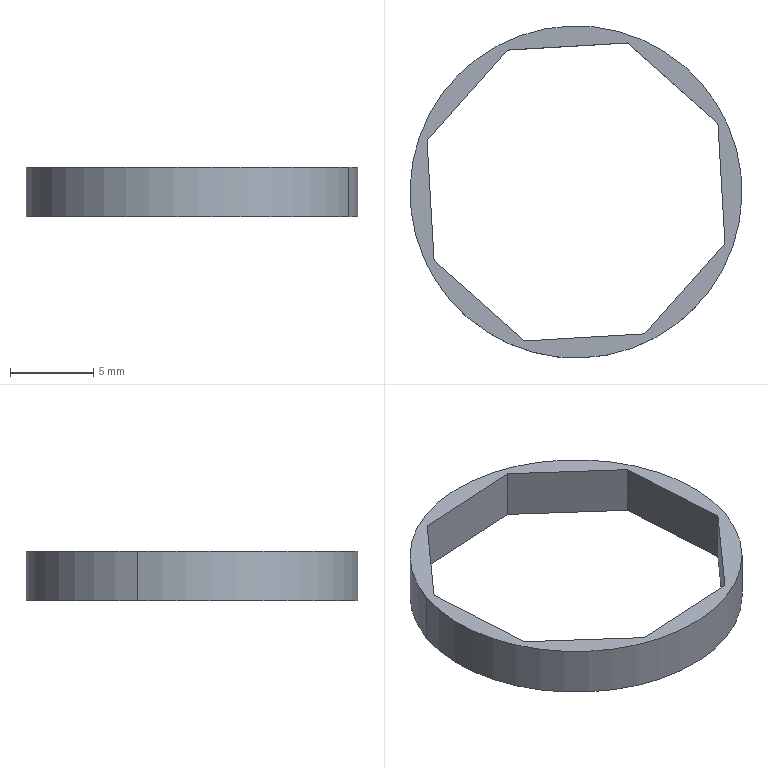Part | SolidWorks | features BaseBody 1 | 1 solid | 12 faces | box 20 x 20 x 3 mm | volume 176.681 mm3 | plane 10 | cylinder 2 | commonest cylinder face diameters 20 x2
STEP:
#1=CARTESIAN_POINT('',(-309.402,-30.274,-448.));
#2=VERTEX_POINT('',#1);
#3=CARTESIAN_POINT('',(-328.298,-23.72,-448.));
#4=VERTEX_POINT('',#3);
#5=CARTESIAN_POINT('',(-318.85,-26.997,-448.));
#6=DIRECTION('',(0.,0.,-1.));
#7=DIRECTION('',(0.9448,-0.3277,0.));
#8=AXIS2_PLACEMENT_3D('',#5,#6,#7);
#9=CIRCLE('',#8,10.);
#10=EDGE_CURVE('',#2,#4,#9,.T.);
#11=ORIENTED_EDGE('',*,*,#10,.F.);
#12=CARTESIAN_POINT('',(-309.402,-30.274,-445.));
#13=VERTEX_POINT('',#12);
#14=CARTESIAN_POINT('',(-309.402,-30.274,-448.));
#15=DIRECTION('',(0.,0.,1.));
#16=VECTOR('',#15,1000.);
#17=LINE('',#14,#16);
#18=EDGE_CURVE('',#2,#13,#17,.T.);
#19=ORIENTED_EDGE('',*,*,#18,.T.);
#20=CARTESIAN_POINT('',(-328.298,-23.72,-445.));
#21=VERTEX_POINT('',#20);
#22=CARTESIAN_POINT('',(-318.85,-26.997,-445.));
#23=DIRECTION('',(0.,0.,-1.));
#24=DIRECTION('',(0.9448,-0.3277,0.));
#25=AXIS2_PLACEMENT_3D('',#22,#23,#24);
#26=CIRCLE('',#25,10.);
#27=EDGE_CURVE('',#13,#21,#26,.T.);
#28=ORIENTED_EDGE('',*,*,#27,.T.);
#29=CARTESIAN_POINT('',(-328.298,-23.72,-448.));
#30=DIRECTION('',(0.,0.,1.));
#31=VECTOR('',#30,1000.);
#32=LINE('',#29,#31);
#33=EDGE_CURVE('',#4,#21,#32,.T.);
#34=ORIENTED_EDGE('',*,*,#33,.F.);
#35=EDGE_LOOP('',(#11,#19,#28,#34));
#36=FACE_OUTER_BOUND('',#35,.T.);
#37=CARTESIAN_POINT('',(-318.85,-26.997,-448.));
#38=DIRECTION('',(0.,0.,1.));
#39=DIRECTION('',(-0.9448,0.3277,0.));
#40=AXIS2_PLACEMENT_3D('',#37,#38,#39);
#41=CYLINDRICAL_SURFACE('',#40,10.);
#42=ADVANCED_FACE('',(#36),#41,.T.);
#43=CARTESIAN_POINT('',(-318.85,-26.997,-448.));
#44=DIRECTION('',(0.,0.,-1.));
#45=DIRECTION('',(0.9448,-0.3277,0.));
#46=AXIS2_PLACEMENT_3D('',#43,#44,#45);
#47=CIRCLE('',#46,10.);
#48=EDGE_CURVE('',#4,#2,#47,.T.);
#49=ORIENTED_EDGE('',*,*,#48,.T.);
#50=ORIENTED_EDGE('',*,*,#10,.T.);
#51=EDGE_LOOP('',(#49,#50));
#52=FACE_OUTER_BOUND('',#51,.T.);
#53=CARTESIAN_POINT('',(-322.995,-18.449,-448.));
#54=VERTEX_POINT('',#53);
#55=CARTESIAN_POINT('',(-315.737,-18.021,-448.));
#56=VERTEX_POINT('',#55);
#57=CARTESIAN_POINT('',(-322.995,-18.449,-448.));
#58=DIRECTION('',(0.9983,0.05883,0.));
#59=VECTOR('',#58,1000.);
#60=LINE('',#57,#59);
#61=EDGE_CURVE('',#54,#56,#60,.T.);
#62=ORIENTED_EDGE('',*,*,#61,.F.);
#63=CARTESIAN_POINT('',(-327.825,-23.884,-448.));
#64=VERTEX_POINT('',#63);
#65=CARTESIAN_POINT('',(-322.995,-18.449,-448.));
#66=DIRECTION('',(0.6643,0.7475,0.));
#67=VECTOR('',#66,1000.);
#68=LINE('',#65,#67);
#69=EDGE_CURVE('',#64,#54,#68,.T.);
#70=ORIENTED_EDGE('',*,*,#69,.F.);
#71=CARTESIAN_POINT('',(-327.398,-31.142,-448.));
#72=VERTEX_POINT('',#71);
#73=CARTESIAN_POINT('',(-327.398,-31.142,-448.));
#74=DIRECTION('',(-0.05883,0.9983,0.));
#75=VECTOR('',#74,1000.);
#76=LINE('',#73,#75);
#77=EDGE_CURVE('',#72,#64,#76,.T.);
#78=ORIENTED_EDGE('',*,*,#77,.F.);
#79=CARTESIAN_POINT('',(-321.963,-35.972,-448.));
#80=VERTEX_POINT('',#79);
#81=CARTESIAN_POINT('',(-327.398,-31.142,-448.));
#82=DIRECTION('',(-0.7475,0.6643,0.));
#83=VECTOR('',#82,1000.);
#84=LINE('',#81,#83);
#85=EDGE_CURVE('',#80,#72,#84,.T.);
#86=ORIENTED_EDGE('',*,*,#85,.F.);
#87=CARTESIAN_POINT('',(-314.704,-35.545,-448.));
#88=VERTEX_POINT('',#87);
#89=CARTESIAN_POINT('',(-314.704,-35.545,-448.));
#90=DIRECTION('',(-0.9983,-0.05883,0.));
#91=VECTOR('',#90,1000.);
#92=LINE('',#89,#91);
#93=EDGE_CURVE('',#88,#80,#92,.T.);
#94=ORIENTED_EDGE('',*,*,#93,.F.);
#95=CARTESIAN_POINT('',(-309.874,-30.11,-448.));
#96=VERTEX_POINT('',#95);
#97=CARTESIAN_POINT('',(-314.704,-35.545,-448.));
#98=DIRECTION('',(-0.6643,-0.7475,0.));
#99=VECTOR('',#98,1000.);
#100=LINE('',#97,#99);
#101=EDGE_CURVE('',#96,#88,#100,.T.);
#102=ORIENTED_EDGE('',*,*,#101,.F.);
#103=CARTESIAN_POINT('',(-310.302,-22.851,-448.));
#104=VERTEX_POINT('',#103);
#105=CARTESIAN_POINT('',(-310.302,-22.851,-448.));
#106=DIRECTION('',(0.05883,-0.9983,0.));
#107=VECTOR('',#106,1000.);
#108=LINE('',#105,#107);
#109=EDGE_CURVE('',#104,#96,#108,.T.);
#110=ORIENTED_EDGE('',*,*,#109,.F.);
#111=CARTESIAN_POINT('',(-310.302,-22.851,-448.));
#112=DIRECTION('',(0.7475,-0.6643,0.));
#113=VECTOR('',#112,1000.);
#114=LINE('',#111,#113);
#115=EDGE_CURVE('',#56,#104,#114,.T.);
#116=ORIENTED_EDGE('',*,*,#115,.F.);
#117=EDGE_LOOP('',(#62,#70,#78,#86,#94,#102,#110,#116));
#118=FACE_BOUND('',#117,.T.);
#119=CARTESIAN_POINT('',(-318.85,-26.997,-448.));
#120=DIRECTION('',(0.,0.,-1.));
#121=DIRECTION('',(0.9448,-0.3277,0.));
#122=AXIS2_PLACEMENT_3D('',#119,#120,#121);
#123=PLANE('',#122);
#124=ADVANCED_FACE('',(#52,#118),#123,.T.);
#125=CARTESIAN_POINT('',(-318.85,-26.997,-445.));
#126=DIRECTION('',(0.,0.,-1.));
#127=DIRECTION('',(0.9448,-0.3277,0.));
#128=AXIS2_PLACEMENT_3D('',#125,#126,#127);
#129=CIRCLE('',#128,10.);
#130=EDGE_CURVE('',#21,#13,#129,.T.);
#131=ORIENTED_EDGE('',*,*,#130,.F.);
#132=ORIENTED_EDGE('',*,*,#27,.F.);
#133=EDGE_LOOP('',(#131,#132));
#134=FACE_OUTER_BOUND('',#133,.T.);
#135=CARTESIAN_POINT('',(-315.737,-18.021,-445.));
#136=VERTEX_POINT('',#135);
#137=CARTESIAN_POINT('',(-310.302,-22.851,-445.));
#138=VERTEX_POINT('',#137);
#139=CARTESIAN_POINT('',(-310.302,-22.851,-445.));
#140=DIRECTION('',(0.7475,-0.6643,0.));
#141=VECTOR('',#140,1000.);
#142=LINE('',#139,#141);
#143=EDGE_CURVE('',#136,#138,#142,.T.);
#144=ORIENTED_EDGE('',*,*,#143,.T.);
#145=CARTESIAN_POINT('',(-309.874,-30.11,-445.));
#146=VERTEX_POINT('',#145);
#147=CARTESIAN_POINT('',(-310.302,-22.851,-445.));
#148=DIRECTION('',(0.05883,-0.9983,0.));
#149=VECTOR('',#148,1000.);
#150=LINE('',#147,#149);
#151=EDGE_CURVE('',#138,#146,#150,.T.);
#152=ORIENTED_EDGE('',*,*,#151,.T.);
#153=CARTESIAN_POINT('',(-314.704,-35.545,-445.));
#154=VERTEX_POINT('',#153);
#155=CARTESIAN_POINT('',(-314.704,-35.545,-445.));
#156=DIRECTION('',(-0.6643,-0.7475,0.));
#157=VECTOR('',#156,1000.);
#158=LINE('',#155,#157);
#159=EDGE_CURVE('',#146,#154,#158,.T.);
#160=ORIENTED_EDGE('',*,*,#159,.T.);
#161=CARTESIAN_POINT('',(-321.963,-35.972,-445.));
#162=VERTEX_POINT('',#161);
#163=CARTESIAN_POINT('',(-314.704,-35.545,-445.));
#164=DIRECTION('',(-0.9983,-0.05883,0.));
#165=VECTOR('',#164,1000.);
#166=LINE('',#163,#165);
#167=EDGE_CURVE('',#154,#162,#166,.T.);
#168=ORIENTED_EDGE('',*,*,#167,.T.);
#169=CARTESIAN_POINT('',(-327.398,-31.142,-445.));
#170=VERTEX_POINT('',#169);
#171=CARTESIAN_POINT('',(-327.398,-31.142,-445.));
#172=DIRECTION('',(-0.7475,0.6643,0.));
#173=VECTOR('',#172,1000.);
#174=LINE('',#171,#173);
#175=EDGE_CURVE('',#162,#170,#174,.T.);
#176=ORIENTED_EDGE('',*,*,#175,.T.);
#177=CARTESIAN_POINT('',(-327.825,-23.884,-445.));
#178=VERTEX_POINT('',#177);
#179=CARTESIAN_POINT('',(-327.398,-31.142,-445.));
#180=DIRECTION('',(-0.05883,0.9983,0.));
#181=VECTOR('',#180,1000.);
#182=LINE('',#179,#181);
#183=EDGE_CURVE('',#170,#178,#182,.T.);
#184=ORIENTED_EDGE('',*,*,#183,.T.);
#185=CARTESIAN_POINT('',(-322.995,-18.449,-445.));
#186=VERTEX_POINT('',#185);
#187=CARTESIAN_POINT('',(-322.995,-18.449,-445.));
#188=DIRECTION('',(0.6643,0.7475,0.));
#189=VECTOR('',#188,1000.);
#190=LINE('',#187,#189);
#191=EDGE_CURVE('',#178,#186,#190,.T.);
#192=ORIENTED_EDGE('',*,*,#191,.T.);
#193=CARTESIAN_POINT('',(-322.995,-18.449,-445.));
#194=DIRECTION('',(0.9983,0.05883,0.));
#195=VECTOR('',#194,1000.);
#196=LINE('',#193,#195);
#197=EDGE_CURVE('',#186,#136,#196,.T.);
#198=ORIENTED_EDGE('',*,*,#197,.T.);
#199=EDGE_LOOP('',(#144,#152,#160,#168,#176,#184,#192,#198));
#200=FACE_BOUND('',#199,.T.);
#201=CARTESIAN_POINT('',(-318.85,-26.997,-445.));
#202=DIRECTION('',(0.,0.,-1.));
#203=DIRECTION('',(0.9448,-0.3277,0.));
#204=AXIS2_PLACEMENT_3D('',#201,#202,#203);
#205=PLANE('',#204);
#206=ADVANCED_FACE('',(#134,#200),#205,.F.);
#207=ORIENTED_EDGE('',*,*,#18,.F.);
#208=ORIENTED_EDGE('',*,*,#48,.F.);
#209=ORIENTED_EDGE('',*,*,#33,.T.);
#210=ORIENTED_EDGE('',*,*,#130,.T.);
#211=EDGE_LOOP('',(#207,#208,#209,#210));
#212=FACE_OUTER_BOUND('',#211,.T.);
#213=CARTESIAN_POINT('',(-318.85,-26.997,-448.));
#214=DIRECTION('',(0.,0.,1.));
#215=DIRECTION('',(-0.9448,0.3277,0.));
#216=AXIS2_PLACEMENT_3D('',#213,#214,#215);
#217=CYLINDRICAL_SURFACE('',#216,10.);
#218=ADVANCED_FACE('',(#212),#217,.T.);
#219=ORIENTED_EDGE('',*,*,#143,.F.);
#220=CARTESIAN_POINT('',(-315.737,-18.021,-448.));
#221=DIRECTION('',(0.,0.,-1.));
#222=VECTOR('',#221,1000.);
#223=LINE('',#220,#222);
#224=EDGE_CURVE('',#136,#56,#223,.T.);
#225=ORIENTED_EDGE('',*,*,#224,.T.);
#226=ORIENTED_EDGE('',*,*,#115,.T.);
#227=CARTESIAN_POINT('',(-310.302,-22.851,-448.));
#228=DIRECTION('',(0.,0.,-1.));
#229=VECTOR('',#228,1000.);
#230=LINE('',#227,#229);
#231=EDGE_CURVE('',#138,#104,#230,.T.);
#232=ORIENTED_EDGE('',*,*,#231,.F.);
#233=EDGE_LOOP('',(#219,#225,#226,#232));
#234=FACE_OUTER_BOUND('',#233,.T.);
#235=CARTESIAN_POINT('',(-310.302,-22.851,-448.));
#236=DIRECTION('',(-0.6643,-0.7475,0.));
#237=DIRECTION('',(0.7475,-0.6643,0.));
#238=AXIS2_PLACEMENT_3D('',#235,#236,#237);
#239=PLANE('',#238);
#240=ADVANCED_FACE('',(#234),#239,.T.);
#241=ORIENTED_EDGE('',*,*,#197,.F.);
#242=CARTESIAN_POINT('',(-322.995,-18.449,-448.));
#243=DIRECTION('',(0.,0.,-1.));
#244=VECTOR('',#243,1000.);
#245=LINE('',#242,#244);
#246=EDGE_CURVE('',#186,#54,#245,.T.);
#247=ORIENTED_EDGE('',*,*,#246,.T.);
#248=ORIENTED_EDGE('',*,*,#61,.T.);
#249=ORIENTED_EDGE('',*,*,#224,.F.);
#250=EDGE_LOOP('',(#241,#247,#248,#249));
#251=FACE_OUTER_BOUND('',#250,.T.);
#252=CARTESIAN_POINT('',(-322.995,-18.449,-448.));
#253=DIRECTION('',(0.05883,-0.9983,0.));
#254=DIRECTION('',(0.9983,0.05883,0.));
#255=AXIS2_PLACEMENT_3D('',#252,#253,#254);
#256=PLANE('',#255);
#257=ADVANCED_FACE('',(#251),#256,.T.);
#258=ORIENTED_EDGE('',*,*,#191,.F.);
#259=CARTESIAN_POINT('',(-327.825,-23.884,-448.));
#260=DIRECTION('',(0.,0.,-1.));
#261=VECTOR('',#260,1000.);
#262=LINE('',#259,#261);
#263=EDGE_CURVE('',#178,#64,#262,.T.);
#264=ORIENTED_EDGE('',*,*,#263,.T.);
#265=ORIENTED_EDGE('',*,*,#69,.T.);
#266=ORIENTED_EDGE('',*,*,#246,.F.);
#267=EDGE_LOOP('',(#258,#264,#265,#266));
#268=FACE_OUTER_BOUND('',#267,.T.);
#269=CARTESIAN_POINT('',(-322.995,-18.449,-448.));
#270=DIRECTION('',(0.7475,-0.6643,0.));
#271=DIRECTION('',(0.6643,0.7475,0.));
#272=AXIS2_PLACEMENT_3D('',#269,#270,#271);
#273=PLANE('',#272);
#274=ADVANCED_FACE('',(#268),#273,.T.);
#275=ORIENTED_EDGE('',*,*,#183,.F.);
#276=CARTESIAN_POINT('',(-327.398,-31.142,-448.));
#277=DIRECTION('',(0.,0.,-1.));
#278=VECTOR('',#277,1000.);
#279=LINE('',#276,#278);
#280=EDGE_CURVE('',#170,#72,#279,.T.);
#281=ORIENTED_EDGE('',*,*,#280,.T.);
#282=ORIENTED_EDGE('',*,*,#77,.T.);
#283=ORIENTED_EDGE('',*,*,#263,.F.);
#284=EDGE_LOOP('',(#275,#281,#282,#283));
#285=FACE_OUTER_BOUND('',#284,.T.);
#286=CARTESIAN_POINT('',(-327.398,-31.142,-448.));
#287=DIRECTION('',(0.9983,0.05883,0.));
#288=DIRECTION('',(-0.05883,0.9983,0.));
#289=AXIS2_PLACEMENT_3D('',#286,#287,#288);
#290=PLANE('',#289);
#291=ADVANCED_FACE('',(#285),#290,.T.);
#292=ORIENTED_EDGE('',*,*,#175,.F.);
#293=CARTESIAN_POINT('',(-321.963,-35.972,-448.));
#294=DIRECTION('',(0.,0.,-1.));
#295=VECTOR('',#294,1000.);
#296=LINE('',#293,#295);
#297=EDGE_CURVE('',#162,#80,#296,.T.);
#298=ORIENTED_EDGE('',*,*,#297,.T.);
#299=ORIENTED_EDGE('',*,*,#85,.T.);
#300=ORIENTED_EDGE('',*,*,#280,.F.);
#301=EDGE_LOOP('',(#292,#298,#299,#300));
#302=FACE_OUTER_BOUND('',#301,.T.);
#303=CARTESIAN_POINT('',(-327.398,-31.142,-448.));
#304=DIRECTION('',(0.6643,0.7475,0.));
#305=DIRECTION('',(-0.7475,0.6643,0.));
#306=AXIS2_PLACEMENT_3D('',#303,#304,#305);
#307=PLANE('',#306);
#308=ADVANCED_FACE('',(#302),#307,.T.);
#309=ORIENTED_EDGE('',*,*,#167,.F.);
#310=CARTESIAN_POINT('',(-314.704,-35.545,-448.));
#311=DIRECTION('',(0.,0.,-1.));
#312=VECTOR('',#311,1000.);
#313=LINE('',#310,#312);
#314=EDGE_CURVE('',#154,#88,#313,.T.);
#315=ORIENTED_EDGE('',*,*,#314,.T.);
#316=ORIENTED_EDGE('',*,*,#93,.T.);
#317=ORIENTED_EDGE('',*,*,#297,.F.);
#318=EDGE_LOOP('',(#309,#315,#316,#317));
#319=FACE_OUTER_BOUND('',#318,.T.);
#320=CARTESIAN_POINT('',(-314.704,-35.545,-448.));
#321=DIRECTION('',(-0.05883,0.9983,0.));
#322=DIRECTION('',(-0.9983,-0.05883,0.));
#323=AXIS2_PLACEMENT_3D('',#320,#321,#322);
#324=PLANE('',#323);
#325=ADVANCED_FACE('',(#319),#324,.T.);
#326=ORIENTED_EDGE('',*,*,#159,.F.);
#327=CARTESIAN_POINT('',(-309.874,-30.11,-448.));
#328=DIRECTION('',(0.,0.,-1.));
#329=VECTOR('',#328,1000.);
#330=LINE('',#327,#329);
#331=EDGE_CURVE('',#146,#96,#330,.T.);
#332=ORIENTED_EDGE('',*,*,#331,.T.);
#333=ORIENTED_EDGE('',*,*,#101,.T.);
#334=ORIENTED_EDGE('',*,*,#314,.F.);
#335=EDGE_LOOP('',(#326,#332,#333,#334));
#336=FACE_OUTER_BOUND('',#335,.T.);
#337=CARTESIAN_POINT('',(-314.704,-35.545,-448.));
#338=DIRECTION('',(-0.7475,0.6643,0.));
#339=DIRECTION('',(-0.6643,-0.7475,0.));
#340=AXIS2_PLACEMENT_3D('',#337,#338,#339);
#341=PLANE('',#340);
#342=ADVANCED_FACE('',(#336),#341,.T.);
#343=ORIENTED_EDGE('',*,*,#151,.F.);
#344=ORIENTED_EDGE('',*,*,#231,.T.);
#345=ORIENTED_EDGE('',*,*,#109,.T.);
#346=ORIENTED_EDGE('',*,*,#331,.F.);
#347=EDGE_LOOP('',(#343,#344,#345,#346));
#348=FACE_OUTER_BOUND('',#347,.T.);
#349=CARTESIAN_POINT('',(-310.302,-22.851,-448.));
#350=DIRECTION('',(-0.9983,-0.05883,0.));
#351=DIRECTION('',(0.05883,-0.9983,0.));
#352=AXIS2_PLACEMENT_3D('',#349,#350,#351);
#353=PLANE('',#352);
#354=ADVANCED_FACE('',(#348),#353,.T.);
#355=CLOSED_SHELL('',(#42,#124,#206,#218,#240,#257,#274,#291,#308,#325,#342,#354));
#356=MANIFOLD_SOLID_BREP('',#355);
#357=CARTESIAN_POINT('',(0.,0.,0.));
#358=DIRECTION('',(0.,0.,1.));
#359=DIRECTION('',(1.,0.,0.));
#360=AXIS2_PLACEMENT_3D('',#357,#358,#359);
#361=(LENGTH_UNIT()NAMED_UNIT(*)SI_UNIT(.MILLI.,.METRE.));
#362=UNCERTAINTY_MEASURE_WITH_UNIT(LENGTH_MEASURE(0.00001),#361,'','');
#363=(NAMED_UNIT(*)PLANE_ANGLE_UNIT()SI_UNIT($,.RADIAN.));
#364=(NAMED_UNIT(*)SI_UNIT($,.STERADIAN.)SOLID_ANGLE_UNIT());
#365=(GEOMETRIC_REPRESENTATION_CONTEXT(3)GLOBAL_UNCERTAINTY_ASSIGNED_CONTEXT((#362))GLOBAL_UNIT_ASSIGNED_CONTEXT((#361,#363,#364))REPRESENTATION_CONTEXT('',''));
#366=ADVANCED_BREP_SHAPE_REPRESENTATION('',(#356,#360),#365);